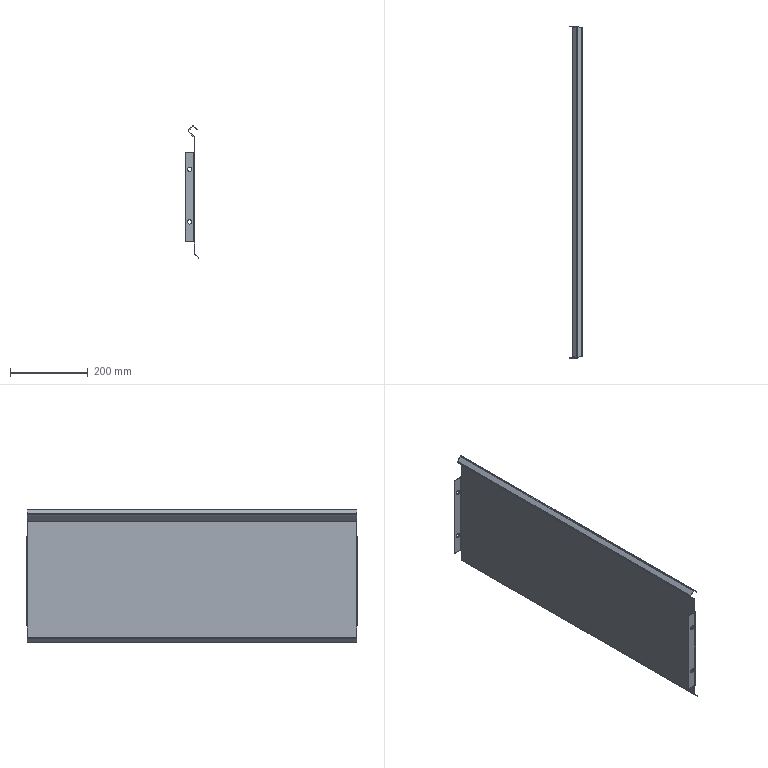Part | SolidWorks | features BaseBody 1 | 1 solid | 50 faces | box 35.167 x 852 x 340.123 mm | volume 484748 mm3 | plane 26 | cylinder 24 | commonest cylinder face diameters 3 x8 6 x8 11 x8